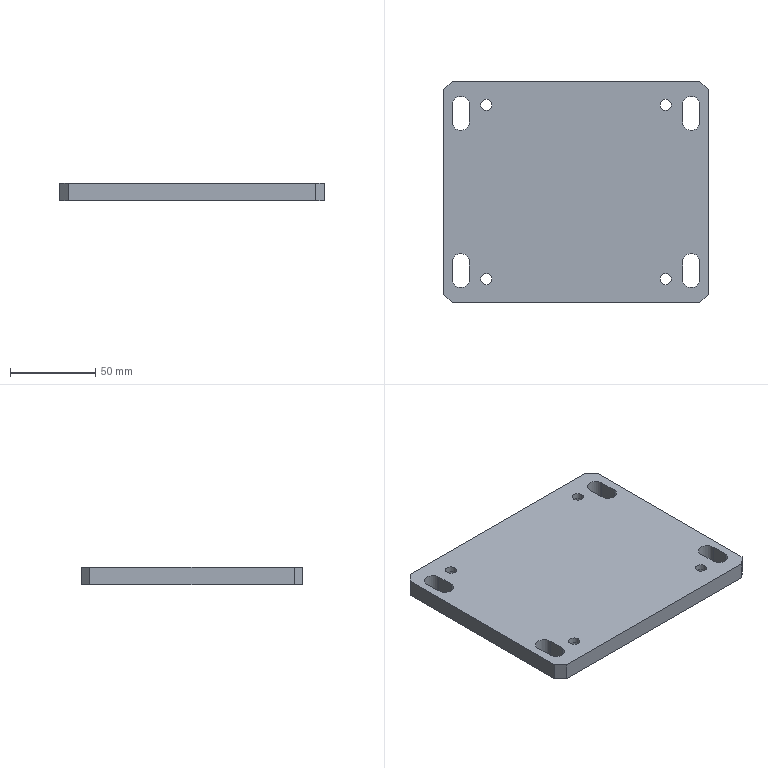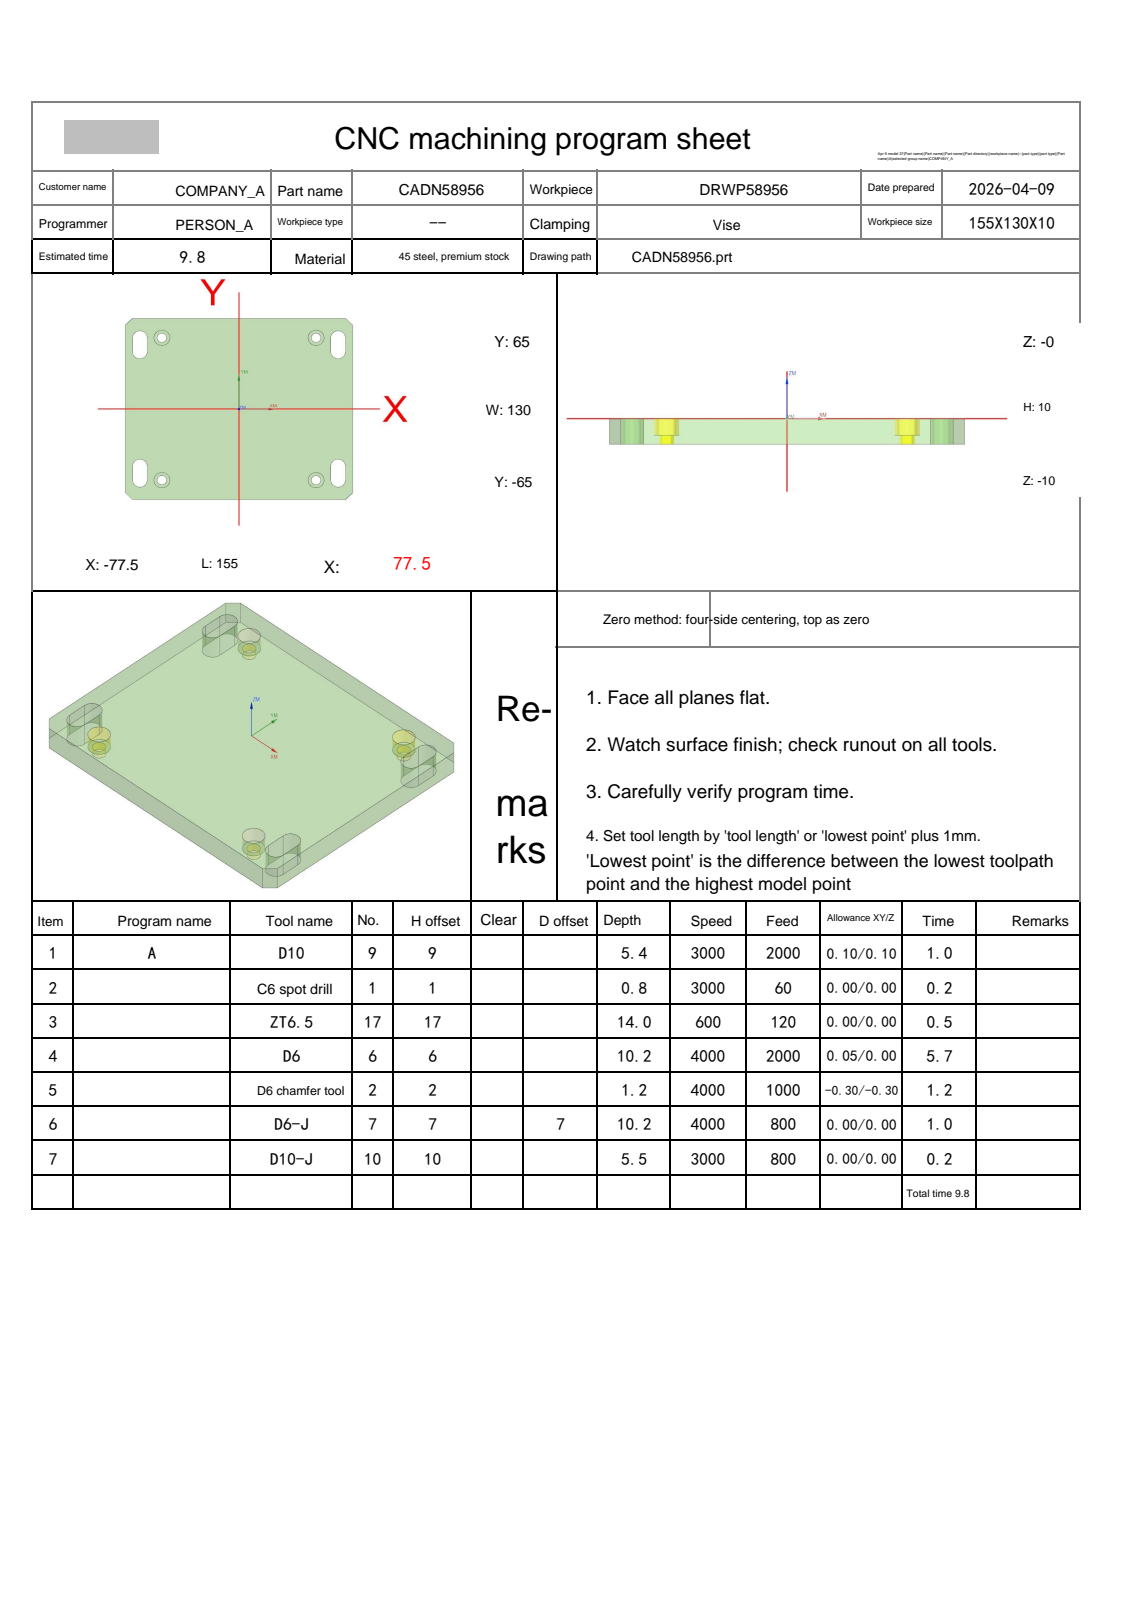NC program | NX | posted by the shop | part box 155 x 130 x 10 mm
Lines 1869 to 2515 of 2515:
N5 T02 M06
(D6 chamfer tool  D=6. R=0. H=02 ce=-0.30 di=0.00)
G00 G90 G54 X50.491 Y-55.357 M03 S4000
G43 H02 Z20.
M08
Z2.5
G01 X50.666 Y-55.439 Z2.43 F800.
X51.101 Y-55.595 Z2.261
X51.55 Y-55.708 Z2.093
X52.007 Y-55.778 Z1.925
X52.469 Y-55.803 Z1.756
X52.931 Y-55.784 Z1.588
X53.39 Y-55.72 Z1.419
X53.84 Y-55.612 Z1.251
X54.277 Y-55.462 Z1.083
X54.698 Y-55.27 Z.914
X55.099 Y-55.039 Z.746
X55.476 Y-54.77 Z.577
X55.825 Y-54.466 Z.409
X56.143 Y-54.13 Z.241
X56.427 Y-53.765 Z.072
X56.675 Y-53.375 Z-.096
X56.884 Y-52.962 Z-.265
X57.052 Y-52.531 Z-.433
X57.179 Y-52.086 Z-.601
X57.261 Y-51.631 Z-.77
X57.3 Y-51.17 Z-.938
Y-51. Z-1.
G03 X52.5 Y-46.2 I-4.8 J0.0
X47.7 Y-51. I0.0 J-4.8
X52.5 Y-55.8 I4.8 J0.0
X57.3 Y-51. I0.0 J4.8
X57.274 Y-50.501 I-4.8 J0.0
G01 Z1.5
G00 Z20.
X50.491 Y46.643
Z2.5
G01 X50.666 Y46.561 Z2.43
X51.101 Y46.405 Z2.261
X51.55 Y46.292 Z2.093
X52.007 Y46.222 Z1.925
X52.469 Y46.197 Z1.756
X52.931 Y46.216 Z1.588
X53.39 Y46.28 Z1.419
X53.84 Y46.388 Z1.251
X54.277 Y46.538 Z1.083
X54.698 Y46.73 Z.914
X55.099 Y46.961 Z.746
X55.476 Y47.23 Z.577
X55.825 Y47.534 Z.409
X56.143 Y47.87 Z.241
X56.427 Y48.235 Z.072
X56.675 Y48.625 Z-.096
X56.884 Y49.038 Z-.265
X57.052 Y49.469 Z-.433
X57.179 Y49.914 Z-.601
X57.261 Y50.369 Z-.77
X57.3 Y50.83 Z-.938
Y51. Z-1.
G03 X52.5 Y55.8 I-4.8 J0.0
X47.7 Y51. I0.0 J-4.8
X52.5 Y46.2 I4.8 J0.0
X57.3 Y51. I0.0 J4.8
X57.274 Y51.499 I-4.8 J0.0
G01 Z1.5
G00 Z20.
X-54.509 Y46.643
Z2.5
G01 X-54.334 Y46.561 Z2.43
X-53.899 Y46.405 Z2.261
X-53.45 Y46.292 Z2.093
X-52.993 Y46.222 Z1.925
X-52.531 Y46.197 Z1.756
X-52.069 Y46.216 Z1.588
X-51.61 Y46.28 Z1.419
X-51.16 Y46.388 Z1.251
X-50.723 Y46.538 Z1.083
X-50.302 Y46.73 Z.914
X-49.901 Y46.961 Z.746
X-49.524 Y47.23 Z.577
X-49.175 Y47.534 Z.409
X-48.857 Y47.87 Z.241
X-48.573 Y48.235 Z.072
X-48.325 Y48.625 Z-.096
X-48.116 Y49.038 Z-.265
X-47.948 Y49.469 Z-.433
X-47.821 Y49.914 Z-.601
X-47.739 Y50.369 Z-.77
X-47.7 Y50.83 Z-.938
Y51. Z-1.
G03 X-52.5 Y55.8 I-4.8 J0.0
X-57.3 Y51. I0.0 J-4.8
X-52.5 Y46.2 I4.8 J0.0
X-47.7 Y51. I0.0 J4.8
X-47.726 Y51.499 I-4.8 J0.0
G01 Z1.5
G00 Z20.
X-54.509 Y-55.357
Z2.5
G01 X-54.334 Y-55.439 Z2.43
X-53.899 Y-55.595 Z2.261
X-53.45 Y-55.708 Z2.093
X-52.993 Y-55.778 Z1.925
X-52.531 Y-55.803 Z1.756
X-52.069 Y-55.784 Z1.588
X-51.61 Y-55.72 Z1.419
X-51.16 Y-55.612 Z1.251
X-50.723 Y-55.462 Z1.083
X-50.302 Y-55.27 Z.914
X-49.901 Y-55.039 Z.746
X-49.524 Y-54.77 Z.577
X-49.175 Y-54.466 Z.409
X-48.857 Y-54.13 Z.241
X-48.573 Y-53.765 Z.072
X-48.325 Y-53.375 Z-.096
X-48.116 Y-52.962 Z-.265
X-47.948 Y-52.531 Z-.433
X-47.821 Y-52.086 Z-.601
X-47.739 Y-51.631 Z-.77
X-47.7 Y-51.17 Z-.938
Y-51. Z-1.
G03 X-52.5 Y-46.2 I-4.8 J0.0
X-57.3 Y-51. I0.0 J-4.8
X-52.5 Y-55.8 I4.8 J0.0
X-47.7 Y-51. I0.0 J4.8
X-47.726 Y-50.501 I-4.8 J0.0
G01 Z1.5
G00 Z20.
G00 G90 X-.386 Y66.227 M03 S3500
Z20.
Z.172
G01 Z-1.2 F1000.
G03 X-.1 Y66.027 I1.286 J1.532
G01 X-.054 Y65.997
X0.0 Y66.
X72.5
X72.759 Y65.966
X73. Y65.866
X73.207 Y65.707
X78.207 Y60.707
X78.366 Y60.5
X78.466 Y60.259
X78.5 Y60.
Y-60.
X78.466 Y-60.259
X78.366 Y-60.5
X78.207 Y-60.707
X73.207 Y-65.707
X73. Y-65.866
X72.759 Y-65.966
X72.5 Y-66.
X-72.5
X-72.759 Y-65.966
X-73. Y-65.866
X-73.207 Y-65.707
X-78.207 Y-60.707
X-78.366 Y-60.5
X-78.466 Y-60.259
X-78.5 Y-60.
Y60.
X-78.466 Y60.259
X-78.366 Y60.5
X-78.207 Y60.707
X-73.207 Y65.707
X-73. Y65.866
X-72.759 Y65.966
X-72.5 Y66.
X0.0
X.054 Y65.997
X.1 Y66.027
G03 X.386 Y66.227 I-1. J1.732
G01 Z.172
G00 Z10.
X-56.799 Y-50.6
Z.219
G01 Z-1.2
G03 X-56.98 Y-50.898 I1.613 J-1.183
G01 X-57.006 Y-50.946
X-57. Y-51.
G03 X-52.5 Y-55.5 I4.5 J0.0
X-48. Y-51. I0.0 J4.5
X-52.5 Y-46.5 I-4.5 J0.0
X-57. Y-51. I0.0 J-4.5
G01 X-57.006 Y-51.054
X-56.98 Y-51.102
G03 X-56.799 Y-51.4 I1.794 J.885
G01 Z.226
G00 Z10.
X-71.273 Y-45.614
Z.172
G01 Z-1.2
G03 X-71.473 Y-45.9 I1.532 J-1.286
G01 X-71.503 Y-45.946
X-71.5 Y-46.
Y-51.
G03 X-67.5 Y-55. I4. J0.0
X-63.5 Y-51. I0.0 J4.
G01 Y-41.
G03 X-67.5 Y-37. I-4. J0.0
X-71.5 Y-41. I0.0 J-4.
G01 Y-46.
X-71.503 Y-46.054
X-71.473 Y-46.1
G03 X-71.273 Y-46.386 I1.732 J1.
G01 Z.172
G00 Z10.
Y46.386
Z.172
G01 Z-1.2
G03 X-71.473 Y46.1 I1.532 J-1.286
G01 X-71.503 Y46.054
X-71.5 Y46.
Y41.
G03 X-67.5 Y37. I4. J0.0
X-63.5 Y41. I0.0 J4.
G01 Y51.
G03 X-67.5 Y55. I-4. J0.0
X-71.5 Y51. I0.0 J-4.
G01 Y46.
X-71.503 Y45.946
X-71.473 Y45.9
G03 X-71.273 Y45.614 I1.732 J1.
G01 Z.172
G00 Z10.
X-56.799 Y51.4
Z.219
G01 Z-1.2
G03 X-56.98 Y51.102 I1.613 J-1.183
G01 X-57.006 Y51.054
X-57. Y51.
G03 X-52.5 Y46.5 I4.5 J0.0
X-48. Y51. I0.0 J4.5
X-52.5 Y55.5 I-4.5 J0.0
X-57. Y51. I0.0 J-4.5
G01 X-57.006 Y50.946
X-56.98 Y50.898
G03 X-56.799 Y50.6 I1.794 J.885
G01 Z.226
G00 Z10.
X48.201 Y51.4
Z.226
G01 Z-1.2
G03 X48.02 Y51.102 I1.613 J-1.183
G01 X47.994 Y51.054
X48. Y51.
G03 X52.5 Y46.5 I4.5 J0.0
X57. Y51. I0.0 J4.5
X52.5 Y55.5 I-4.5 J0.0
X48. Y51. I0.0 J-4.5
G01 X47.994 Y50.946
X48.02 Y50.898
G03 X48.201 Y50.6 I1.794 J.885
G01 Z.219
G00 Z10.
X63.727 Y46.386
Z.172
G01 Z-1.2
G03 X63.527 Y46.1 I1.532 J-1.286
G01 X63.497 Y46.054
X63.5 Y46.
Y41.
G03 X67.5 Y37. I4. J0.0
X71.5 Y41. I0.0 J4.
G01 Y51.
G03 X67.5 Y55. I-4. J0.0
X63.5 Y51. I0.0 J-4.
G01 Y46.
X63.497 Y45.946
X63.527 Y45.9
G03 X63.727 Y45.614 I1.732 J1.
G01 Z.172
G00 Z10.
Y-45.614
Z.172
G01 Z-1.2
G03 X63.527 Y-45.9 I1.532 J-1.286
G01 X63.497 Y-45.946
X63.5 Y-46.
Y-51.
G03 X67.5 Y-55. I4. J0.0
X71.5 Y-51. I0.0 J4.
G01 Y-41.
G03 X67.5 Y-37. I-4. J0.0
X63.5 Y-41. I0.0 J-4.
G01 Y-46.
X63.497 Y-46.054
X63.527 Y-46.1
G03 X63.727 Y-46.386 I1.732 J1.
G01 Z.172
G00 Z10.
X48.201 Y-50.6
Z.226
G01 Z-1.2
G03 X48.02 Y-50.898 I1.613 J-1.183
G01 X47.994 Y-50.946
X48. Y-51.
G03 X52.5 Y-55.5 I4.5 J0.0
X57. Y-51. I0.0 J4.5
X52.5 Y-46.5 I-4.5 J0.0
X48. Y-51. I0.0 J-4.5
G01 X47.994 Y-51.054
X48.02 Y-51.102
G03 X48.201 Y-51.4 I1.794 J.885
G01 Z.219
G00 Z20.
G91 G28 Z0.0
M05
M09
G91 G28 Z0.0
M01
N6 T07 M06
(D6-J  D=6. R=0. H=07 ce=0.00 di=0.00)
G00 G90 G54 X-52.5 Y-51. M03 S4000
G43 H07 Z20.
M08
Z0.0
G41 D07
G01 X-52.468 Y-51.197 F800.
G03 X-51.242 Y-52.242 I1.226 J.197
X-50. Y-51. I0.0 J1.242
X-50. Y-51. Z-5. I-2.5 J0.0
X-53.273 Y-48.622 Z-6.5 I-2.5 J0.0
X-55. Y-51. I.773 J-2.378
X-52.5 Y-53.5 I2.5 J0.0
X-50. Y-51. I0.0 J2.5
X-52.5 Y-48.5 I-2.5 J0.0
X-53.273 Y-48.622 I0.0 J-2.5
X-54.131 Y-49.804 I.384 J-1.181
X-52.889 Y-51.046 I1.242 J0.0
G01 X-52.698 Y-51.031
G40 X-52.5 Y-51.
G00 Z20.
X52.5 Y51.
Z0.0
G41 D07
G01 X52.532 Y50.803
G03 X53.758 Y49.758 I1.226 J.197
X55. Y51. I0.0 J1.242
X55. Y51. Z-5. I-2.5 J0.0
X51.727 Y53.378 Z-6.5 I-2.5 J0.0
X50. Y51. I.773 J-2.378
X52.5 Y48.5 I2.5 J0.0
X55. Y51. I0.0 J2.5
X52.5 Y53.5 I-2.5 J0.0
X51.727 Y53.378 I0.0 J-2.5
X50.869 Y52.196 I.384 J-1.181
X52.111 Y50.954 I1.242 J0.0
G01 X52.302 Y50.969
G40 X52.5 Y51.
G00 Z20.
G00 G90 X52.5 Y-51. M03 S4000
Z20.
Z0.0
G41 D07
G01 X52.532 Y-51.197 F800.
G03 X53.758 Y-52.242 I1.226 J.197
X55. Y-51. I0.0 J1.242
X55. Y-51. Z-5. I-2.5 J0.0
X51.727 Y-48.622 Z-6.5 I-2.5 J0.0
X50. Y-51. I.773 J-2.378
X52.5 Y-53.5 I2.5 J0.0
X55. Y-51. I0.0 J2.5
X52.5 Y-48.5 I-2.5 J0.0
X51.727 Y-48.622 I0.0 J-2.5
X50.869 Y-49.804 I.384 J-1.181
X52.111 Y-51.046 I1.242 J0.0
G01 X52.302 Y-51.031
G40 X52.5 Y-51.
G00 Z20.
X-52.5 Y51.
Z0.0
G41 D07
G01 X-52.468 Y50.803
G03 X-51.242 Y49.758 I1.226 J.197
X-50. Y51. I0.0 J1.242
X-50. Y51. Z-5. I-2.5 J0.0
X-53.273 Y53.378 Z-6.5 I-2.5 J0.0
X-55. Y51. I.773 J-2.378
X-52.5 Y48.5 I2.5 J0.0
X-50. Y51. I0.0 J2.5
X-52.5 Y53.5 I-2.5 J0.0
X-53.273 Y53.378 I0.0 J-2.5
X-54.131 Y52.196 I.384 J-1.181
X-52.889 Y50.954 I1.242 J0.0
G01 X-52.698 Y50.969
G40 X-52.5 Y51.
G00 Z20.
G00 G90 X65.535 Y-47.604 M03 S3500
Z20.
Z.5
G01 Y-51.14 Z.315 F800.
X65.591 Y-51.487 Z.296
X65.708 Y-51.818 Z.278
X65.882 Y-52.123 Z.259
X66.107 Y-52.393 Z.241
X66.377 Y-52.618 Z.223
X66.682 Y-52.792 Z.204
X67.013 Y-52.909 Z.186
X67.36 Y-52.965 Z.167
X67.64 Z.153
X68.031 Y-52.897 Z.132
X68.4 Y-52.753 Z.111
X68.732 Y-52.537 Z.09
X69.015 Y-52.26 Z.07
X69.236 Y-51.931 Z.049
X69.387 Y-51.565 Z.028
X69.462 Y-51.176 Z.007
X69.465 Y-51.035 Z0.0
G41 D07
X69.5 Y-51.
Y-41. Z-1.044
G03 X67.5 Y-39. Z-1.372 I-2. J0.0
X65.5 Y-41. Z-1.7 I0.0 J-2.
G01 Y-51. Z-2.744
G03 X67.5 Y-53. Z-3.072 I2. J0.0
X69.5 Y-51. Z-3.4 I0.0 J2.
G01 Y-41. Z-4.444
G03 X67.5 Y-39. Z-4.772 I-2. J0.0
X65.5 Y-41. Z-5.1 I0.0 J-2.
G01 Y-51. Z-6.144
G03 X67.5 Y-53. Z-6.472 I2. J0.0
X69.5 Y-51. Z-6.8 I0.0 J2.
G01 Y-41. Z-7.844
G03 X67.5 Y-39. Z-8.172 I-2. J0.0
X65.5 Y-41. Z-8.5 I0.0 J-2.
G01 Y-51. Z-9.544
G03 X67.5 Y-53. Z-9.872 I2. J0.0
X69.5 Y-51. Z-10.2 I0.0 J2.
G01 Y-41.
G03 X67.5 Y-39. I-2. J0.0
X65.5 Y-41. I0.0 J-2.
G01 Y-51.
G03 X67.5 Y-53. I2. J0.0
X69.5 Y-51. I0.0 J2.
G01 Y-50.6
X69.498 Y-50.573
X69.478 Y-50.552
X69.45 Y-50.55
G40 X69.4
Z-9.2
G00 Z20.
X65.535 Y44.396
Z.5
G01 Y40.86 Z.315
X65.591 Y40.513 Z.296
X65.708 Y40.182 Z.278
X65.882 Y39.877 Z.259
X66.107 Y39.607 Z.241
X66.377 Y39.382 Z.223
X66.682 Y39.208 Z.204
X67.013 Y39.091 Z.186
X67.36 Y39.035 Z.167
X67.64 Z.153
X68.031 Y39.103 Z.132
X68.4 Y39.247 Z.111
X68.732 Y39.463 Z.09
X69.015 Y39.74 Z.07
X69.236 Y40.069 Z.049
X69.387 Y40.435 Z.028
X69.462 Y40.824 Z.007
X69.465 Y40.965 Z0.0
G41 D07
X69.5 Y41.
Y51. Z-1.044
G03 X67.5 Y53. Z-1.372 I-2. J0.0
X65.5 Y51. Z-1.7 I0.0 J-2.
G01 Y41. Z-2.744
G03 X67.5 Y39. Z-3.072 I2. J0.0
X69.5 Y41. Z-3.4 I0.0 J2.
G01 Y51. Z-4.444
G03 X67.5 Y53. Z-4.772 I-2. J0.0
X65.5 Y51. Z-5.1 I0.0 J-2.
G01 Y41. Z-6.144
G03 X67.5 Y39. Z-6.472 I2. J0.0
X69.5 Y41. Z-6.8 I0.0 J2.
G01 Y51. Z-7.844
G03 X67.5 Y53. Z-8.172 I-2. J0.0
X65.5 Y51. Z-8.5 I0.0 J-2.
G01 Y41. Z-9.544
G03 X67.5 Y39. Z-9.872 I2. J0.0
X69.5 Y41. Z-10.2 I0.0 J2.
G01 Y51.
G03 X67.5 Y53. I-2. J0.0
X65.5 Y51. I0.0 J-2.
G01 Y41.
G03 X67.5 Y39. I2. J0.0
X69.5 Y41. I0.0 J2.
G01 Y41.4
X69.498 Y41.428
X69.478 Y41.448
X69.45 Y41.45
G40 X69.4
Z-9.2
G00 Z20.
X-65.535 Y47.604
Z.5
G01 Y51.14 Z.315
X-65.591 Y51.487 Z.296
X-65.708 Y51.818 Z.278
X-65.882 Y52.123 Z.259
X-66.107 Y52.393 Z.241
X-66.377 Y52.618 Z.223
X-66.682 Y52.792 Z.204
X-67.013 Y52.909 Z.186
X-67.36 Y52.965 Z.167
X-67.64 Z.153
X-68.031 Y52.897 Z.132
X-68.4 Y52.753 Z.111
X-68.732 Y52.537 Z.09
X-69.015 Y52.26 Z.07
X-69.236 Y51.931 Z.049
X-69.387 Y51.565 Z.028
X-69.462 Y51.176 Z.007
X-69.465 Y51.035 Z0.0
G41 D07
X-69.5 Y51.
Y41. Z-1.044
G03 X-67.5 Y39. Z-1.372 I2. J0.0
X-65.5 Y41. Z-1.7 I0.0 J2.
G01 Y51. Z-2.744
G03 X-67.5 Y53. Z-3.072 I-2. J0.0
X-69.5 Y51. Z-3.4 I0.0 J-2.
G01 Y41. Z-4.444
G03 X-67.5 Y39. Z-4.772 I2. J0.0
X-65.5 Y41. Z-5.1 I0.0 J2.
G01 Y51. Z-6.144
G03 X-67.5 Y53. Z-6.472 I-2. J0.0
X-69.5 Y51. Z-6.8 I0.0 J-2.
G01 Y41. Z-7.844
G03 X-67.5 Y39. Z-8.172 I2. J0.0
X-65.5 Y41. Z-8.5 I0.0 J2.
G01 Y51. Z-9.544
G03 X-67.5 Y53. Z-9.872 I-2. J0.0
X-69.5 Y51. Z-10.2 I0.0 J-2.
G01 Y41.
G03 X-67.5 Y39. I2. J0.0
X-65.5 Y41. I0.0 J2.
G01 Y51.
G03 X-67.5 Y53. I-2. J0.0
X-69.5 Y51. I0.0 J-2.
G01 Y50.6
X-69.498 Y50.573
X-69.478 Y50.552
X-69.45 Y50.55
G40 X-69.4
Z-9.2
G00 Z20.
X-65.535 Y-44.396
Z.5
G01 Y-40.86 Z.315
X-65.591 Y-40.513 Z.296
X-65.708 Y-40.182 Z.278
X-65.882 Y-39.877 Z.259
X-66.107 Y-39.607 Z.241
X-66.377 Y-39.382 Z.223
X-66.682 Y-39.208 Z.204
X-67.013 Y-39.091 Z.186
X-67.36 Y-39.035 Z.167
X-67.64 Z.153
X-68.031 Y-39.103 Z.132
X-68.4 Y-39.247 Z.111
X-68.732 Y-39.463 Z.09
X-69.015 Y-39.74 Z.07
X-69.236 Y-40.069 Z.049
X-69.387 Y-40.435 Z.028
X-69.462 Y-40.824 Z.007
X-69.465 Y-40.965 Z0.0
G41 D07
X-69.5 Y-41.
Y-51. Z-1.044
G03 X-67.5 Y-53. Z-1.372 I2. J0.0
X-65.5 Y-51. Z-1.7 I0.0 J2.
G01 Y-41. Z-2.744
G03 X-67.5 Y-39. Z-3.072 I-2. J0.0
X-69.5 Y-41. Z-3.4 I0.0 J-2.
G01 Y-51. Z-4.444
G03 X-67.5 Y-53. Z-4.772 I2. J0.0
X-65.5 Y-51. Z-5.1 I0.0 J2.
G01 Y-41. Z-6.144
G03 X-67.5 Y-39. Z-6.472 I-2. J0.0
X-69.5 Y-41. Z-6.8 I0.0 J-2.
G01 Y-51. Z-7.844
G03 X-67.5 Y-53. Z-8.172 I2. J0.0
X-65.5 Y-51. Z-8.5 I0.0 J2.
G01 Y-41. Z-9.544
G03 X-67.5 Y-39. Z-9.872 I-2. J0.0
X-69.5 Y-41. Z-10.2 I0.0 J-2.
G01 Y-51.
G03 X-67.5 Y-53. I2. J0.0
X-65.5 Y-51. I0.0 J2.
G01 Y-41.
G03 X-67.5 Y-39. I-2. J0.0
X-69.5 Y-41. I0.0 J-2.
G01 Y-41.4
X-69.498 Y-41.428
X-69.478 Y-41.448
X-69.45 Y-41.45
G40 X-69.4
Z-9.2
G00 Z20.
G91 G28 Z0.0
M05
M09
G91 G28 Z0.0
M01
N7 T10 M06
(D10-J  D=10. R=0. H=10 ce=0.00 di=0.00)
G00 G90 G54 X-71.793 Y-72.778 M03 S3000
G43 H10 Z20.
M08
Z-4.5
G01 Z-5.5 F800.
X-76.036 Y-68.536
X-81.036 Y-63.536
X-85.278 Y-59.293
Z-4.5
G00 Z20.
Y59.293
Z-4.5
G01 Z-5.5
X-81.036 Y63.536
X-76.036 Y68.536
X-71.793 Y72.778
Z-4.5
G00 Z20.
X71.793
Z-4.5
G01 Z-5.5
X76.036 Y68.536
X81.036 Y63.536
X85.278 Y59.293
Z-4.5
G00 Z20.
Y-59.293
Z-4.5
G01 Z-5.5
X81.036 Y-63.536
X76.036 Y-68.536
X71.793 Y-72.778
Z-4.5
G00 Z20.
M05
M09
G91 G28 Z0.0
G91 G28 Y0.0
M30
%